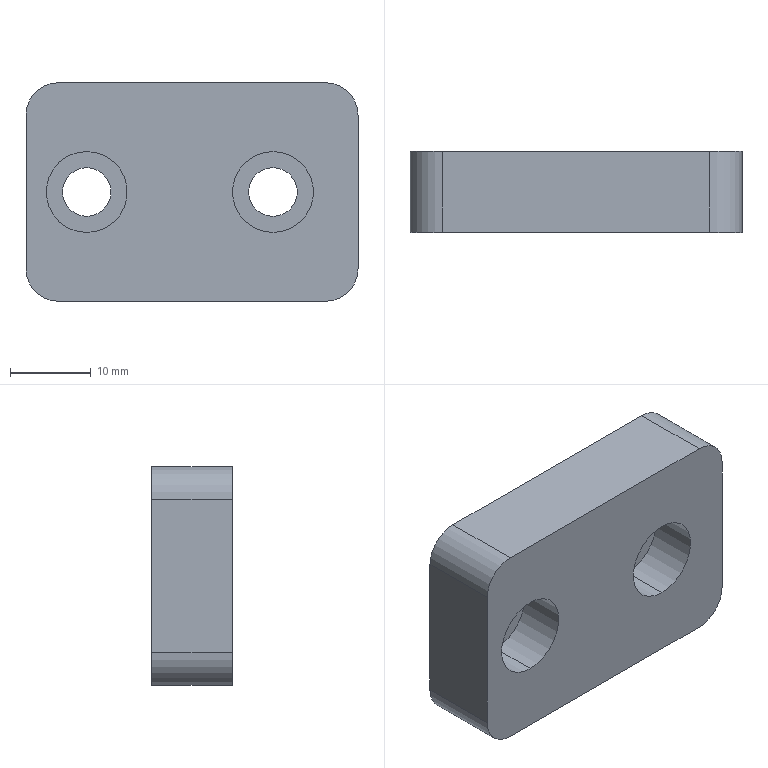Part | STEP file | 1 solid | 20 faces | box 41 x 10 x 27 mm | volume 9764 mm3 | cylinder 12 | plane 8 | commonest cylinder face diameters 6 x4 8 x4 10 x4